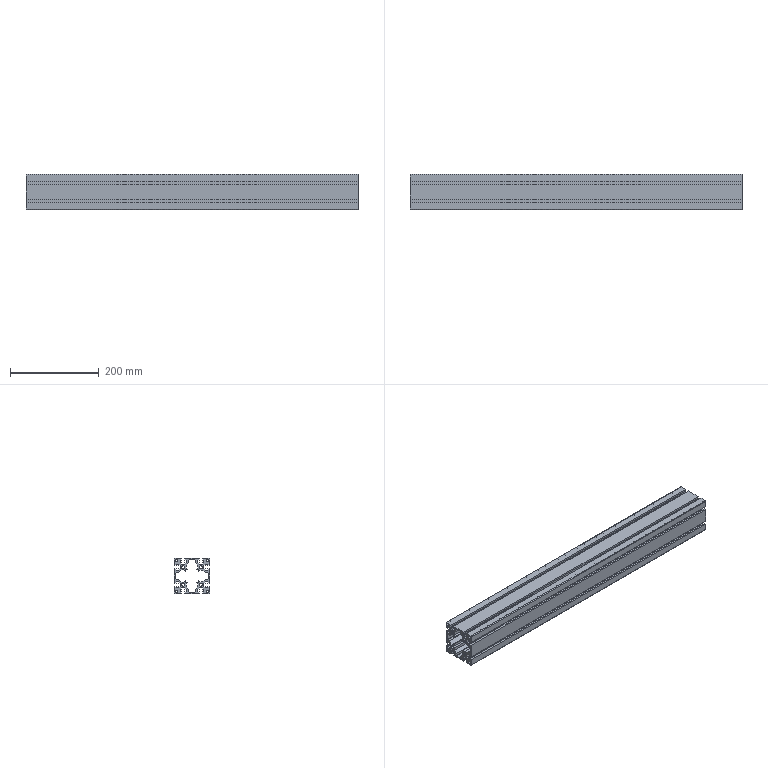Part | SolidWorks | features ICE 1, WeldMemberFeat 1, WeldmentFeature 1 | 1 solid | 174 faces | box 750 x 80 x 80 mm | volume 1716766 mm3 | plane 146 | cylinder 28 | commonest cylinder face diameters 2 x8 6 x8 6.8 x8 3 x4